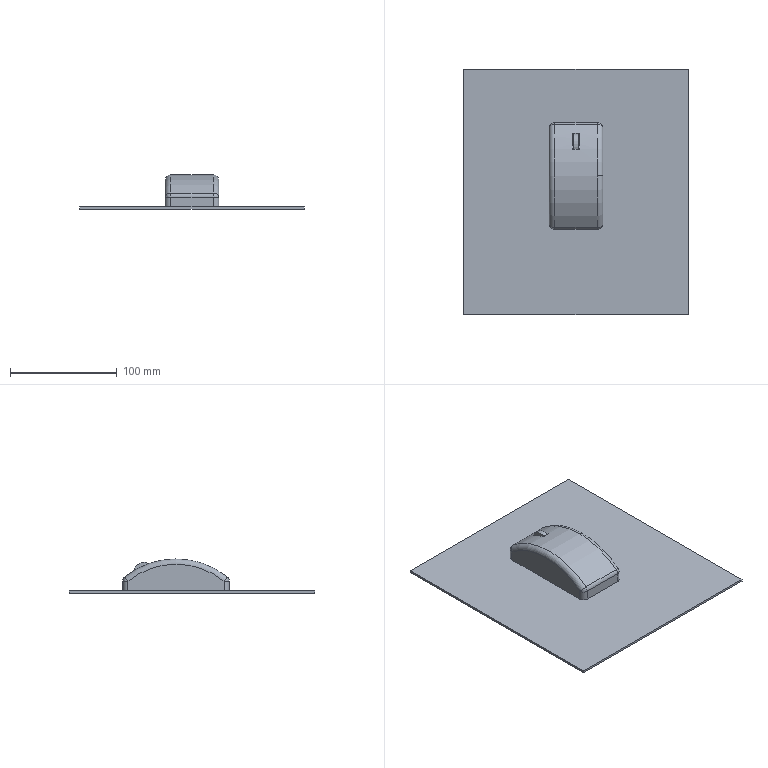Part | SolidWorks | features ICE 4, Fillet 2, Extrusion 1 | 1 solid | 32 faces | box 210 x 230 x 32 mm | volume 215921 mm3 | plane 17 | cylinder 8 | sphere 4 | torus 3 | commonest cylinder face diameters 10 x6 21 x1 153.572 x1
STEP:
#1=CARTESIAN_POINT('',(50.,50.,25.));
#2=VERTEX_POINT('',#1);
#3=CARTESIAN_POINT('',(50.,5.,9.145));
#4=VERTEX_POINT('',#3);
#5=CARTESIAN_POINT('',(50.,50.,-46.786));
#6=DIRECTION('',(1.,0.,0.));
#7=DIRECTION('',(0.,0.,1.));
#8=AXIS2_PLACEMENT_3D('',#5,#6,#7);
#9=CIRCLE('',#8,71.786);
#10=EDGE_CURVE('',#2,#4,#9,.T.);
#11=ORIENTED_EDGE('',*,*,#10,.F.);
#12=CARTESIAN_POINT('',(45.,50.,30.));
#13=VERTEX_POINT('',#12);
#14=CARTESIAN_POINT('',(45.,50.,25.));
#15=DIRECTION('',(0.,-1.,0.));
#16=DIRECTION('',(0.,0.,-1.));
#17=AXIS2_PLACEMENT_3D('',#14,#15,#16);
#18=CIRCLE('',#17,5.);
#19=EDGE_CURVE('',#2,#13,#18,.T.);
#20=ORIENTED_EDGE('',*,*,#19,.T.);
#21=CARTESIAN_POINT('',(45.,1.866,13.04));
#22=VERTEX_POINT('',#21);
#23=CARTESIAN_POINT('',(45.,50.,-46.786));
#24=DIRECTION('',(-1.,0.,0.));
#25=DIRECTION('',(0.,0.,1.));
#26=AXIS2_PLACEMENT_3D('',#23,#24,#25);
#27=CIRCLE('',#26,76.786);
#28=EDGE_CURVE('',#22,#13,#27,.T.);
#29=ORIENTED_EDGE('',*,*,#28,.F.);
#30=CARTESIAN_POINT('',(45.,5.,9.145));
#31=DIRECTION('',(0.,0.7791,0.6269));
#32=DIRECTION('',(0.,-0.6269,0.7791));
#33=AXIS2_PLACEMENT_3D('',#30,#31,#32);
#34=CIRCLE('',#33,5.);
#35=EDGE_CURVE('',#22,#4,#34,.T.);
#36=ORIENTED_EDGE('',*,*,#35,.T.);
#37=EDGE_LOOP('',(#11,#20,#29,#36));
#38=FACE_OUTER_BOUND('',#37,.T.);
#39=CARTESIAN_POINT('',(45.,50.,-46.786));
#40=DIRECTION('',(-1.,0.,0.));
#41=DIRECTION('',(0.,0.,1.));
#42=AXIS2_PLACEMENT_3D('',#39,#40,#41);
#43=TOROIDAL_SURFACE('',#42,71.786,5.);
#44=ADVANCED_FACE('',(#38),#43,.T.);
#45=CARTESIAN_POINT('',(23.,75.,25.703));
#46=VERTEX_POINT('',#45);
#47=CARTESIAN_POINT('',(27.,75.,25.703));
#48=VERTEX_POINT('',#47);
#49=CARTESIAN_POINT('',(23.,75.,25.703));
#50=DIRECTION('',(1.,0.,0.));
#51=VECTOR('',#50,1000.);
#52=LINE('',#49,#51);
#53=EDGE_CURVE('',#46,#48,#52,.T.);
#54=ORIENTED_EDGE('',*,*,#53,.F.);
#55=CARTESIAN_POINT('',(23.,75.,16.45));
#56=VERTEX_POINT('',#55);
#57=CARTESIAN_POINT('',(23.,75.,26.45));
#58=DIRECTION('',(0.,0.,-1.));
#59=VECTOR('',#58,1000.);
#60=LINE('',#57,#59);
#61=EDGE_CURVE('',#46,#56,#60,.T.);
#62=ORIENTED_EDGE('',*,*,#61,.T.);
#63=CARTESIAN_POINT('',(22.,75.,16.45));
#64=VERTEX_POINT('',#63);
#65=CARTESIAN_POINT('',(28.,75.,16.45));
#66=DIRECTION('',(-1.,0.,0.));
#67=VECTOR('',#66,1000.);
#68=LINE('',#65,#67);
#69=EDGE_CURVE('',#56,#64,#68,.T.);
#70=ORIENTED_EDGE('',*,*,#69,.T.);
#71=CARTESIAN_POINT('',(22.,75.,25.816));
#72=VERTEX_POINT('',#71);
#73=CARTESIAN_POINT('',(22.,75.,26.45));
#74=DIRECTION('',(0.,0.,-1.));
#75=VECTOR('',#74,1000.);
#76=LINE('',#73,#75);
#77=EDGE_CURVE('',#72,#64,#76,.T.);
#78=ORIENTED_EDGE('',*,*,#77,.F.);
#79=CARTESIAN_POINT('',(28.,75.,25.816));
#80=VERTEX_POINT('',#79);
#81=CARTESIAN_POINT('',(0.,75.,25.816));
#82=DIRECTION('',(1.,0.,0.));
#83=VECTOR('',#82,1000.);
#84=LINE('',#81,#83);
#85=EDGE_CURVE('',#72,#80,#84,.T.);
#86=ORIENTED_EDGE('',*,*,#85,.T.);
#87=CARTESIAN_POINT('',(28.,75.,16.45));
#88=VERTEX_POINT('',#87);
#89=CARTESIAN_POINT('',(28.,75.,26.45));
#90=DIRECTION('',(0.,0.,-1.));
#91=VECTOR('',#90,1000.);
#92=LINE('',#89,#91);
#93=EDGE_CURVE('',#80,#88,#92,.T.);
#94=ORIENTED_EDGE('',*,*,#93,.T.);
#95=CARTESIAN_POINT('',(27.,75.,16.45));
#96=VERTEX_POINT('',#95);
#97=CARTESIAN_POINT('',(28.,75.,16.45));
#98=DIRECTION('',(-1.,0.,0.));
#99=VECTOR('',#98,1000.);
#100=LINE('',#97,#99);
#101=EDGE_CURVE('',#88,#96,#100,.T.);
#102=ORIENTED_EDGE('',*,*,#101,.T.);
#103=CARTESIAN_POINT('',(27.,75.,26.45));
#104=DIRECTION('',(0.,0.,-1.));
#105=VECTOR('',#104,1000.);
#106=LINE('',#103,#105);
#107=EDGE_CURVE('',#48,#96,#106,.T.);
#108=ORIENTED_EDGE('',*,*,#107,.F.);
#109=EDGE_LOOP('',(#54,#62,#70,#78,#86,#94,#102,#108));
#110=FACE_OUTER_BOUND('',#109,.T.);
#111=CARTESIAN_POINT('',(28.,75.,26.45));
#112=DIRECTION('',(0.,1.,0.));
#113=DIRECTION('',(0.,0.,1.));
#114=AXIS2_PLACEMENT_3D('',#111,#112,#113);
#115=PLANE('',#114);
#116=ADVANCED_FACE('',(#110),#115,.T.);
#117=ORIENTED_EDGE('',*,*,#69,.F.);
#118=CARTESIAN_POINT('',(23.,89.997,16.45));
#119=VERTEX_POINT('',#118);
#120=CARTESIAN_POINT('',(23.,90.,16.45));
#121=DIRECTION('',(0.,1.,0.));
#122=VECTOR('',#121,1000.);
#123=LINE('',#120,#122);
#124=EDGE_CURVE('',#56,#119,#123,.T.);
#125=ORIENTED_EDGE('',*,*,#124,.T.);
#126=CARTESIAN_POINT('',(27.,89.997,16.45));
#127=VERTEX_POINT('',#126);
#128=CARTESIAN_POINT('',(23.,89.997,16.45));
#129=DIRECTION('',(-1.,0.,0.));
#130=VECTOR('',#129,1000.);
#131=LINE('',#128,#130);
#132=EDGE_CURVE('',#127,#119,#131,.T.);
#133=ORIENTED_EDGE('',*,*,#132,.F.);
#134=CARTESIAN_POINT('',(27.,90.,16.45));
#135=DIRECTION('',(0.,1.,0.));
#136=VECTOR('',#135,1000.);
#137=LINE('',#134,#136);
#138=EDGE_CURVE('',#96,#127,#137,.T.);
#139=ORIENTED_EDGE('',*,*,#138,.F.);
#140=ORIENTED_EDGE('',*,*,#101,.F.);
#141=CARTESIAN_POINT('',(28.,90.,16.45));
#142=VERTEX_POINT('',#141);
#143=CARTESIAN_POINT('',(28.,90.,16.45));
#144=DIRECTION('',(0.,1.,0.));
#145=VECTOR('',#144,1000.);
#146=LINE('',#143,#145);
#147=EDGE_CURVE('',#88,#142,#146,.T.);
#148=ORIENTED_EDGE('',*,*,#147,.T.);
#149=CARTESIAN_POINT('',(22.,90.,16.45));
#150=VERTEX_POINT('',#149);
#151=CARTESIAN_POINT('',(28.,90.,16.45));
#152=DIRECTION('',(-1.,0.,0.));
#153=VECTOR('',#152,1000.);
#154=LINE('',#151,#153);
#155=EDGE_CURVE('',#142,#150,#154,.T.);
#156=ORIENTED_EDGE('',*,*,#155,.T.);
#157=CARTESIAN_POINT('',(22.,90.,16.45));
#158=DIRECTION('',(0.,1.,0.));
#159=VECTOR('',#158,1000.);
#160=LINE('',#157,#159);
#161=EDGE_CURVE('',#64,#150,#160,.T.);
#162=ORIENTED_EDGE('',*,*,#161,.F.);
#163=EDGE_LOOP('',(#117,#125,#133,#139,#140,#148,#156,#162));
#164=FACE_OUTER_BOUND('',#163,.T.);
#165=CARTESIAN_POINT('',(28.,90.,16.45));
#166=DIRECTION('',(0.,0.,1.));
#167=DIRECTION('',(1.,0.,0.));
#168=AXIS2_PLACEMENT_3D('',#165,#166,#167);
#169=PLANE('',#168);
#170=ADVANCED_FACE('',(#164),#169,.T.);
#171=CARTESIAN_POINT('',(0.,5.,9.145));
#172=VERTEX_POINT('',#171);
#173=CARTESIAN_POINT('',(0.,95.,9.145));
#174=VERTEX_POINT('',#173);
#175=CARTESIAN_POINT('',(0.,50.,-46.786));
#176=DIRECTION('',(-1.,0.,0.));
#177=DIRECTION('',(0.,0.,-1.));
#178=AXIS2_PLACEMENT_3D('',#175,#176,#177);
#179=CIRCLE('',#178,71.786);
#180=EDGE_CURVE('',#172,#174,#179,.T.);
#181=ORIENTED_EDGE('',*,*,#180,.T.);
#182=CARTESIAN_POINT('',(0.,95.,0.));
#183=VERTEX_POINT('',#182);
#184=CARTESIAN_POINT('',(0.,95.,30.));
#185=DIRECTION('',(0.,0.,-1.));
#186=VECTOR('',#185,1000.);
#187=LINE('',#184,#186);
#188=EDGE_CURVE('',#174,#183,#187,.T.);
#189=ORIENTED_EDGE('',*,*,#188,.T.);
#190=CARTESIAN_POINT('',(0.,5.,0.));
#191=VERTEX_POINT('',#190);
#192=CARTESIAN_POINT('',(0.,0.,0.));
#193=DIRECTION('',(0.,-1.,0.));
#194=VECTOR('',#193,1000.);
#195=LINE('',#192,#194);
#196=EDGE_CURVE('',#183,#191,#195,.T.);
#197=ORIENTED_EDGE('',*,*,#196,.T.);
#198=CARTESIAN_POINT('',(0.,5.,30.));
#199=DIRECTION('',(0.,0.,1.));
#200=VECTOR('',#199,1000.);
#201=LINE('',#198,#200);
#202=EDGE_CURVE('',#191,#172,#201,.T.);
#203=ORIENTED_EDGE('',*,*,#202,.T.);
#204=EDGE_LOOP('',(#181,#189,#197,#203));
#205=FACE_OUTER_BOUND('',#204,.T.);
#206=CARTESIAN_POINT('',(0.,0.,30.));
#207=DIRECTION('',(1.,0.,0.));
#208=DIRECTION('',(0.,0.,-1.));
#209=AXIS2_PLACEMENT_3D('',#206,#207,#208);
#210=PLANE('',#209);
#211=ADVANCED_FACE('',(#205),#210,.F.);
#212=CARTESIAN_POINT('',(5.,0.,0.));
#213=VERTEX_POINT('',#212);
#214=CARTESIAN_POINT('',(45.,0.,0.));
#215=VERTEX_POINT('',#214);
#216=CARTESIAN_POINT('',(0.,0.,0.));
#217=DIRECTION('',(1.,0.,0.));
#218=VECTOR('',#217,1000.);
#219=LINE('',#216,#218);
#220=EDGE_CURVE('',#213,#215,#219,.T.);
#221=ORIENTED_EDGE('',*,*,#220,.T.);
#222=CARTESIAN_POINT('',(45.,0.,9.145));
#223=VERTEX_POINT('',#222);
#224=CARTESIAN_POINT('',(45.,0.,30.));
#225=DIRECTION('',(0.,0.,1.));
#226=VECTOR('',#225,1000.);
#227=LINE('',#224,#226);
#228=EDGE_CURVE('',#215,#223,#227,.T.);
#229=ORIENTED_EDGE('',*,*,#228,.T.);
#230=CARTESIAN_POINT('',(5.,0.,9.145));
#231=VERTEX_POINT('',#230);
#232=CARTESIAN_POINT('',(0.,0.,9.145));
#233=DIRECTION('',(-1.,0.,0.));
#234=VECTOR('',#233,1000.);
#235=LINE('',#232,#234);
#236=EDGE_CURVE('',#223,#231,#235,.T.);
#237=ORIENTED_EDGE('',*,*,#236,.T.);
#238=CARTESIAN_POINT('',(5.,0.,30.));
#239=DIRECTION('',(0.,0.,-1.));
#240=VECTOR('',#239,1000.);
#241=LINE('',#238,#240);
#242=EDGE_CURVE('',#231,#213,#241,.T.);
#243=ORIENTED_EDGE('',*,*,#242,.T.);
#244=EDGE_LOOP('',(#221,#229,#237,#243));
#245=FACE_OUTER_BOUND('',#244,.T.);
#246=CARTESIAN_POINT('',(0.,0.,30.));
#247=DIRECTION('',(0.,1.,0.));
#248=DIRECTION('',(0.,0.,1.));
#249=AXIS2_PLACEMENT_3D('',#246,#247,#248);
#250=PLANE('',#249);
#251=ADVANCED_FACE('',(#245),#250,.F.);
#252=CARTESIAN_POINT('',(50.,5.,0.));
#253=VERTEX_POINT('',#252);
#254=CARTESIAN_POINT('',(50.,95.,0.));
#255=VERTEX_POINT('',#254);
#256=CARTESIAN_POINT('',(50.,0.,0.));
#257=DIRECTION('',(0.,1.,0.));
#258=VECTOR('',#257,1000.);
#259=LINE('',#256,#258);
#260=EDGE_CURVE('',#253,#255,#259,.T.);
#261=ORIENTED_EDGE('',*,*,#260,.T.);
#262=CARTESIAN_POINT('',(50.,95.,9.145));
#263=VERTEX_POINT('',#262);
#264=CARTESIAN_POINT('',(50.,95.,30.));
#265=DIRECTION('',(0.,0.,1.));
#266=VECTOR('',#265,1000.);
#267=LINE('',#264,#266);
#268=EDGE_CURVE('',#255,#263,#267,.T.);
#269=ORIENTED_EDGE('',*,*,#268,.T.);
#270=CARTESIAN_POINT('',(50.,50.,-46.786));
#271=DIRECTION('',(1.,0.,0.));
#272=DIRECTION('',(0.,0.,1.));
#273=AXIS2_PLACEMENT_3D('',#270,#271,#272);
#274=CIRCLE('',#273,71.786);
#275=EDGE_CURVE('',#263,#2,#274,.T.);
#276=ORIENTED_EDGE('',*,*,#275,.T.);
#277=ORIENTED_EDGE('',*,*,#10,.T.);
#278=CARTESIAN_POINT('',(50.,5.,30.));
#279=DIRECTION('',(0.,0.,-1.));
#280=VECTOR('',#279,1000.);
#281=LINE('',#278,#280);
#282=EDGE_CURVE('',#4,#253,#281,.T.);
#283=ORIENTED_EDGE('',*,*,#282,.T.);
#284=EDGE_LOOP('',(#261,#269,#276,#277,#283));
#285=FACE_OUTER_BOUND('',#284,.T.);
#286=CARTESIAN_POINT('',(50.,0.,30.));
#287=DIRECTION('',(-1.,0.,0.));
#288=DIRECTION('',(0.,0.,1.));
#289=AXIS2_PLACEMENT_3D('',#286,#287,#288);
#290=PLANE('',#289);
#291=ADVANCED_FACE('',(#285),#290,.F.);
#292=CARTESIAN_POINT('',(45.,100.,0.));
#293=VERTEX_POINT('',#292);
#294=CARTESIAN_POINT('',(5.,100.,0.));
#295=VERTEX_POINT('',#294);
#296=CARTESIAN_POINT('',(0.,100.,0.));
#297=DIRECTION('',(-1.,0.,0.));
#298=VECTOR('',#297,1000.);
#299=LINE('',#296,#298);
#300=EDGE_CURVE('',#293,#295,#299,.T.);
#301=ORIENTED_EDGE('',*,*,#300,.T.);
#302=CARTESIAN_POINT('',(5.,100.,9.145));
#303=VERTEX_POINT('',#302);
#304=CARTESIAN_POINT('',(5.,100.,30.));
#305=DIRECTION('',(0.,0.,1.));
#306=VECTOR('',#305,1000.);
#307=LINE('',#304,#306);
#308=EDGE_CURVE('',#295,#303,#307,.T.);
#309=ORIENTED_EDGE('',*,*,#308,.T.);
#310=CARTESIAN_POINT('',(45.,100.,9.145));
#311=VERTEX_POINT('',#310);
#312=CARTESIAN_POINT('',(0.,100.,9.145));
#313=DIRECTION('',(1.,0.,0.));
#314=VECTOR('',#313,1000.);
#315=LINE('',#312,#314);
#316=EDGE_CURVE('',#303,#311,#315,.T.);
#317=ORIENTED_EDGE('',*,*,#316,.T.);
#318=CARTESIAN_POINT('',(45.,100.,30.));
#319=DIRECTION('',(0.,0.,-1.));
#320=VECTOR('',#319,1000.);
#321=LINE('',#318,#320);
#322=EDGE_CURVE('',#311,#293,#321,.T.);
#323=ORIENTED_EDGE('',*,*,#322,.T.);
#324=EDGE_LOOP('',(#301,#309,#317,#323));
#325=FACE_OUTER_BOUND('',#324,.T.);
#326=CARTESIAN_POINT('',(0.,100.,30.));
#327=DIRECTION('',(0.,-1.,0.));
#328=DIRECTION('',(0.,0.,-1.));
#329=AXIS2_PLACEMENT_3D('',#326,#327,#328);
#330=PLANE('',#329);
#331=ADVANCED_FACE('',(#325),#330,.F.);
#332=CARTESIAN_POINT('',(5.,98.134,13.04));
#333=VERTEX_POINT('',#332);
#334=CARTESIAN_POINT('',(5.,1.866,13.04));
#335=VERTEX_POINT('',#334);
#336=CARTESIAN_POINT('',(5.,50.,-46.786));
#337=DIRECTION('',(1.,0.,0.));
#338=DIRECTION('',(0.,0.,-1.));
#339=AXIS2_PLACEMENT_3D('',#336,#337,#338);
#340=CIRCLE('',#339,76.786);
#341=EDGE_CURVE('',#333,#335,#340,.T.);
#342=ORIENTED_EDGE('',*,*,#341,.T.);
#343=CARTESIAN_POINT('',(0.,1.866,13.04));
#344=DIRECTION('',(1.,0.,0.));
#345=VECTOR('',#344,1000.);
#346=LINE('',#343,#345);
#347=EDGE_CURVE('',#335,#22,#346,.T.);
#348=ORIENTED_EDGE('',*,*,#347,.T.);
#349=ORIENTED_EDGE('',*,*,#28,.T.);
#350=CARTESIAN_POINT('',(45.,98.134,13.04));
#351=VERTEX_POINT('',#350);
#352=CARTESIAN_POINT('',(45.,50.,-46.786));
#353=DIRECTION('',(-1.,0.,0.));
#354=DIRECTION('',(0.,0.,1.));
#355=AXIS2_PLACEMENT_3D('',#352,#353,#354);
#356=CIRCLE('',#355,76.786);
#357=EDGE_CURVE('',#13,#351,#356,.T.);
#358=ORIENTED_EDGE('',*,*,#357,.T.);
#359=CARTESIAN_POINT('',(0.,98.134,13.04));
#360=DIRECTION('',(-1.,0.,0.));
#361=VECTOR('',#360,1000.);
#362=LINE('',#359,#361);
#363=EDGE_CURVE('',#351,#333,#362,.T.);
#364=ORIENTED_EDGE('',*,*,#363,.T.);
#365=EDGE_LOOP('',(#342,#348,#349,#358,#364));
#366=FACE_OUTER_BOUND('',#365,.T.);
#367=CARTESIAN_POINT('',(28.,90.,18.759));
#368=VERTEX_POINT('',#367);
#369=CARTESIAN_POINT('',(22.,90.,18.759));
#370=VERTEX_POINT('',#369);
#371=CARTESIAN_POINT('',(0.,90.,18.759));
#372=DIRECTION('',(-1.,0.,0.));
#373=VECTOR('',#372,1000.);
#374=LINE('',#371,#373);
#375=EDGE_CURVE('',#368,#370,#374,.T.);
#376=ORIENTED_EDGE('',*,*,#375,.F.);
#377=CARTESIAN_POINT('',(28.,50.,-46.786));
#378=DIRECTION('',(1.,0.,0.));
#379=DIRECTION('',(0.,0.,-1.));
#380=AXIS2_PLACEMENT_3D('',#377,#378,#379);
#381=CIRCLE('',#380,76.786);
#382=EDGE_CURVE('',#368,#80,#381,.T.);
#383=ORIENTED_EDGE('',*,*,#382,.T.);
#384=ORIENTED_EDGE('',*,*,#85,.F.);
#385=CARTESIAN_POINT('',(22.,50.,-46.786));
#386=DIRECTION('',(1.,0.,0.));
#387=DIRECTION('',(0.,0.,-1.));
#388=AXIS2_PLACEMENT_3D('',#385,#386,#387);
#389=CIRCLE('',#388,76.786);
#390=EDGE_CURVE('',#370,#72,#389,.T.);
#391=ORIENTED_EDGE('',*,*,#390,.F.);
#392=EDGE_LOOP('',(#376,#383,#384,#391));
#393=FACE_BOUND('',#392,.T.);
#394=CARTESIAN_POINT('',(0.,50.,-46.786));
#395=DIRECTION('',(1.,0.,0.));
#396=DIRECTION('',(0.,0.,-1.));
#397=AXIS2_PLACEMENT_3D('',#394,#395,#396);
#398=CYLINDRICAL_SURFACE('',#397,76.786);
#399=ADVANCED_FACE('',(#366,#393),#398,.T.);
#400=ORIENTED_EDGE('',*,*,#375,.T.);
#401=CARTESIAN_POINT('',(22.,90.,26.45));
#402=DIRECTION('',(0.,0.,1.));
#403=VECTOR('',#402,1000.);
#404=LINE('',#401,#403);
#405=EDGE_CURVE('',#150,#370,#404,.T.);
#406=ORIENTED_EDGE('',*,*,#405,.F.);
#407=ORIENTED_EDGE('',*,*,#155,.F.);
#408=CARTESIAN_POINT('',(28.,90.,26.45));
#409=DIRECTION('',(0.,0.,1.));
#410=VECTOR('',#409,1000.);
#411=LINE('',#408,#410);
#412=EDGE_CURVE('',#142,#368,#411,.T.);
#413=ORIENTED_EDGE('',*,*,#412,.T.);
#414=EDGE_LOOP('',(#400,#406,#407,#413));
#415=FACE_OUTER_BOUND('',#414,.T.);
#416=CARTESIAN_POINT('',(28.,90.,26.45));
#417=DIRECTION('',(0.,-1.,0.));
#418=DIRECTION('',(0.,0.,-1.));
#419=AXIS2_PLACEMENT_3D('',#416,#417,#418);
#420=PLANE('',#419);
#421=ADVANCED_FACE('',(#415),#420,.T.);
#422=ORIENTED_EDGE('',*,*,#412,.F.);
#423=ORIENTED_EDGE('',*,*,#147,.F.);
#424=ORIENTED_EDGE('',*,*,#93,.F.);
#425=ORIENTED_EDGE('',*,*,#382,.F.);
#426=EDGE_LOOP('',(#422,#423,#424,#425));
#427=FACE_OUTER_BOUND('',#426,.T.);
#428=CARTESIAN_POINT('',(28.,75.,26.45));
#429=DIRECTION('',(1.,0.,0.));
#430=DIRECTION('',(0.,0.,-1.));
#431=AXIS2_PLACEMENT_3D('',#428,#429,#430);
#432=PLANE('',#431);
#433=ADVANCED_FACE('',(#427),#432,.F.);
#434=ORIENTED_EDGE('',*,*,#390,.T.);
#435=ORIENTED_EDGE('',*,*,#77,.T.);
#436=ORIENTED_EDGE('',*,*,#161,.T.);
#437=ORIENTED_EDGE('',*,*,#405,.T.);
#438=EDGE_LOOP('',(#434,#435,#436,#437));
#439=FACE_OUTER_BOUND('',#438,.T.);
#440=CARTESIAN_POINT('',(22.,75.,26.45));
#441=DIRECTION('',(1.,0.,0.));
#442=DIRECTION('',(0.,0.,-1.));
#443=AXIS2_PLACEMENT_3D('',#440,#441,#442);
#444=PLANE('',#443);
#445=ADVANCED_FACE('',(#439),#444,.T.);
#446=CARTESIAN_POINT('',(23.,79.5,16.217));
#447=DIRECTION('',(1.,0.,0.));
#448=DIRECTION('',(0.,0.,-1.));
#449=AXIS2_PLACEMENT_3D('',#446,#447,#448);
#450=CIRCLE('',#449,10.5);
#451=EDGE_CURVE('',#119,#46,#450,.T.);
#452=ORIENTED_EDGE('',*,*,#451,.T.);
#453=ORIENTED_EDGE('',*,*,#53,.T.);
#454=CARTESIAN_POINT('',(27.,79.5,16.217));
#455=DIRECTION('',(1.,0.,0.));
#456=DIRECTION('',(0.,0.,-1.));
#457=AXIS2_PLACEMENT_3D('',#454,#455,#456);
#458=CIRCLE('',#457,10.5);
#459=EDGE_CURVE('',#127,#48,#458,.T.);
#460=ORIENTED_EDGE('',*,*,#459,.F.);
#461=ORIENTED_EDGE('',*,*,#132,.T.);
#462=EDGE_LOOP('',(#452,#453,#460,#461));
#463=FACE_OUTER_BOUND('',#462,.T.);
#464=CARTESIAN_POINT('',(23.,79.5,16.217));
#465=DIRECTION('',(1.,0.,0.));
#466=DIRECTION('',(0.,0.,-1.));
#467=AXIS2_PLACEMENT_3D('',#464,#465,#466);
#468=CYLINDRICAL_SURFACE('',#467,10.5);
#469=ADVANCED_FACE('',(#463),#468,.T.);
#470=ORIENTED_EDGE('',*,*,#61,.F.);
#471=ORIENTED_EDGE('',*,*,#451,.F.);
#472=ORIENTED_EDGE('',*,*,#124,.F.);
#473=EDGE_LOOP('',(#470,#471,#472));
#474=FACE_OUTER_BOUND('',#473,.T.);
#475=CARTESIAN_POINT('',(23.,79.5,16.217));
#476=DIRECTION('',(1.,0.,0.));
#477=DIRECTION('',(0.,0.,-1.));
#478=AXIS2_PLACEMENT_3D('',#475,#476,#477);
#479=PLANE('',#478);
#480=ADVANCED_FACE('',(#474),#479,.F.);
#481=ORIENTED_EDGE('',*,*,#459,.T.);
#482=ORIENTED_EDGE('',*,*,#107,.T.);
#483=ORIENTED_EDGE('',*,*,#138,.T.);
#484=EDGE_LOOP('',(#481,#482,#483));
#485=FACE_OUTER_BOUND('',#484,.T.);
#486=CARTESIAN_POINT('',(27.,79.5,16.217));
#487=DIRECTION('',(1.,0.,0.));
#488=DIRECTION('',(0.,0.,-1.));
#489=AXIS2_PLACEMENT_3D('',#486,#487,#488);
#490=PLANE('',#489);
#491=ADVANCED_FACE('',(#485),#490,.T.);
#492=ORIENTED_EDGE('',*,*,#316,.F.);
#493=CARTESIAN_POINT('',(5.,95.,9.145));
#494=DIRECTION('',(1.,0.,0.));
#495=DIRECTION('',(0.,0.,-1.));
#496=AXIS2_PLACEMENT_3D('',#493,#494,#495);
#497=CIRCLE('',#496,5.);
#498=EDGE_CURVE('',#303,#333,#497,.T.);
#499=ORIENTED_EDGE('',*,*,#498,.T.);
#500=ORIENTED_EDGE('',*,*,#363,.F.);
#501=CARTESIAN_POINT('',(45.,95.,9.145));
#502=DIRECTION('',(-1.,0.,0.));
#503=DIRECTION('',(0.,0.,-1.));
#504=AXIS2_PLACEMENT_3D('',#501,#502,#503);
#505=CIRCLE('',#504,5.);
#506=EDGE_CURVE('',#351,#311,#505,.T.);
#507=ORIENTED_EDGE('',*,*,#506,.T.);
#508=EDGE_LOOP('',(#492,#499,#500,#507));
#509=FACE_OUTER_BOUND('',#508,.T.);
#510=CARTESIAN_POINT('',(0.,95.,9.145));
#511=DIRECTION('',(1.,0.,0.));
#512=DIRECTION('',(0.,0.,-1.));
#513=AXIS2_PLACEMENT_3D('',#510,#511,#512);
#514=CYLINDRICAL_SURFACE('',#513,5.);
#515=ADVANCED_FACE('',(#509),#514,.T.);
#516=ORIENTED_EDGE('',*,*,#19,.F.);
#517=ORIENTED_EDGE('',*,*,#275,.F.);
#518=CARTESIAN_POINT('',(45.,95.,9.145));
#519=DIRECTION('',(0.,-0.7791,0.6269));
#520=DIRECTION('',(0.,0.6269,0.7791));
#521=AXIS2_PLACEMENT_3D('',#518,#519,#520);
#522=CIRCLE('',#521,5.);
#523=EDGE_CURVE('',#263,#351,#522,.T.);
#524=ORIENTED_EDGE('',*,*,#523,.T.);
#525=ORIENTED_EDGE('',*,*,#357,.F.);
#526=EDGE_LOOP('',(#516,#517,#524,#525));
#527=FACE_OUTER_BOUND('',#526,.T.);
#528=CARTESIAN_POINT('',(45.,50.,-46.786));
#529=DIRECTION('',(-1.,0.,0.));
#530=DIRECTION('',(0.,0.,1.));
#531=AXIS2_PLACEMENT_3D('',#528,#529,#530);
#532=TOROIDAL_SURFACE('',#531,71.786,5.);
#533=ADVANCED_FACE('',(#527),#532,.T.);
#534=ORIENTED_EDGE('',*,*,#341,.F.);
#535=CARTESIAN_POINT('',(5.,95.,9.145));
#536=DIRECTION('',(0.,-0.7791,0.6269));
#537=DIRECTION('',(0.,-0.6269,-0.7791));
#538=AXIS2_PLACEMENT_3D('',#535,#536,#537);
#539=CIRCLE('',#538,5.);
#540=EDGE_CURVE('',#333,#174,#539,.T.);
#541=ORIENTED_EDGE('',*,*,#540,.T.);
#542=ORIENTED_EDGE('',*,*,#180,.F.);
#543=CARTESIAN_POINT('',(5.,5.,9.145));
#544=DIRECTION('',(0.,0.7791,0.6269));
#545=DIRECTION('',(0.,0.6269,-0.7791));
#546=AXIS2_PLACEMENT_3D('',#543,#544,#545);
#547=CIRCLE('',#546,5.);
#548=EDGE_CURVE('',#172,#335,#547,.T.);
#549=ORIENTED_EDGE('',*,*,#548,.T.);
#550=EDGE_LOOP('',(#534,#541,#542,#549));
#551=FACE_OUTER_BOUND('',#550,.T.);
#552=CARTESIAN_POINT('',(5.,50.,-46.786));
#553=DIRECTION('',(1.,0.,0.));
#554=DIRECTION('',(0.,0.,-1.));
#555=AXIS2_PLACEMENT_3D('',#552,#553,#554);
#556=TOROIDAL_SURFACE('',#555,71.786,5.);
#557=ADVANCED_FACE('',(#551),#556,.T.);
#558=ORIENTED_EDGE('',*,*,#236,.F.);
#559=CARTESIAN_POINT('',(45.,5.,9.145));
#560=DIRECTION('',(-1.,0.,0.));
#561=DIRECTION('',(0.,0.,-1.));
#562=AXIS2_PLACEMENT_3D('',#559,#560,#561);
#563=CIRCLE('',#562,5.);
#564=EDGE_CURVE('',#223,#22,#563,.T.);
#565=ORIENTED_EDGE('',*,*,#564,.T.);
#566=ORIENTED_EDGE('',*,*,#347,.F.);
#567=CARTESIAN_POINT('',(5.,5.,9.145));
#568=DIRECTION('',(1.,0.,0.));
#569=DIRECTION('',(0.,0.,-1.));
#570=AXIS2_PLACEMENT_3D('',#567,#568,#569);
#571=CIRCLE('',#570,5.);
#572=EDGE_CURVE('',#335,#231,#571,.T.);
#573=ORIENTED_EDGE('',*,*,#572,.T.);
#574=EDGE_LOOP('',(#558,#565,#566,#573));
#575=FACE_OUTER_BOUND('',#574,.T.);
#576=CARTESIAN_POINT('',(0.,5.,9.145));
#577=DIRECTION('',(1.,0.,0.));
#578=DIRECTION('',(0.,0.,-1.));
#579=AXIS2_PLACEMENT_3D('',#576,#577,#578);
#580=CYLINDRICAL_SURFACE('',#579,5.);
#581=ADVANCED_FACE('',(#575),#580,.T.);
#582=CARTESIAN_POINT('',(5.,95.,9.145));
#583=DIRECTION('',(0.,0.,1.));
#584=DIRECTION('',(1.,0.,0.));
#585=AXIS2_PLACEMENT_3D('',#582,#583,#584);
#586=CIRCLE('',#585,5.);
#587=EDGE_CURVE('',#303,#174,#586,.T.);
#588=ORIENTED_EDGE('',*,*,#587,.F.);
#589=ORIENTED_EDGE('',*,*,#308,.F.);
#590=CARTESIAN_POINT('',(5.,95.,0.));
#591=DIRECTION('',(0.,0.,-1.));
#592=DIRECTION('',(-1.,0.,0.));
#593=AXIS2_PLACEMENT_3D('',#590,#591,#592);
#594=CIRCLE('',#593,5.);
#595=EDGE_CURVE('',#183,#295,#594,.T.);
#596=ORIENTED_EDGE('',*,*,#595,.F.);
#597=ORIENTED_EDGE('',*,*,#188,.F.);
#598=EDGE_LOOP('',(#588,#589,#596,#597));
#599=FACE_OUTER_BOUND('',#598,.T.);
#600=CARTESIAN_POINT('',(5.,95.,30.));
#601=DIRECTION('',(0.,0.,-1.));
#602=DIRECTION('',(-1.,0.,0.));
#603=AXIS2_PLACEMENT_3D('',#600,#601,#602);
#604=CYLINDRICAL_SURFACE('',#603,5.);
#605=ADVANCED_FACE('',(#599),#604,.T.);
#606=ORIENTED_EDGE('',*,*,#540,.F.);
#607=ORIENTED_EDGE('',*,*,#498,.F.);
#608=ORIENTED_EDGE('',*,*,#587,.T.);
#609=EDGE_LOOP('',(#606,#607,#608));
#610=FACE_OUTER_BOUND('',#609,.T.);
#611=CARTESIAN_POINT('',(5.,95.,9.145));
#612=DIRECTION('',(0.,1.,0.));
#613=DIRECTION('',(1.,0.,0.));
#614=AXIS2_PLACEMENT_3D('',#611,#612,#613);
#615=SPHERICAL_SURFACE('',#614,5.);
#616=ADVANCED_FACE('',(#610),#615,.T.);
#617=CARTESIAN_POINT('',(45.,95.,9.145));
#618=DIRECTION('',(0.,0.,1.));
#619=DIRECTION('',(1.,0.,0.));
#620=AXIS2_PLACEMENT_3D('',#617,#618,#619);
#621=CIRCLE('',#620,5.);
#622=EDGE_CURVE('',#263,#311,#621,.T.);
#623=ORIENTED_EDGE('',*,*,#622,.F.);
#624=ORIENTED_EDGE('',*,*,#268,.F.);
#625=CARTESIAN_POINT('',(45.,95.,0.));
#626=DIRECTION('',(0.,0.,-1.));
#627=DIRECTION('',(-1.,0.,0.));
#628=AXIS2_PLACEMENT_3D('',#625,#626,#627);
#629=CIRCLE('',#628,5.);
#630=EDGE_CURVE('',#293,#255,#629,.T.);
#631=ORIENTED_EDGE('',*,*,#630,.F.);
#632=ORIENTED_EDGE('',*,*,#322,.F.);
#633=EDGE_LOOP('',(#623,#624,#631,#632));
#634=FACE_OUTER_BOUND('',#633,.T.);
#635=CARTESIAN_POINT('',(45.,95.,30.));
#636=DIRECTION('',(0.,0.,-1.));
#637=DIRECTION('',(-1.,0.,0.));
#638=AXIS2_PLACEMENT_3D('',#635,#636,#637);
#639=CYLINDRICAL_SURFACE('',#638,5.);
#640=ADVANCED_FACE('',(#634),#639,.T.);
#641=ORIENTED_EDGE('',*,*,#622,.T.);
#642=ORIENTED_EDGE('',*,*,#506,.F.);
#643=ORIENTED_EDGE('',*,*,#523,.F.);
#644=EDGE_LOOP('',(#641,#642,#643));
#645=FACE_OUTER_BOUND('',#644,.T.);
#646=CARTESIAN_POINT('',(45.,95.,9.145));
#647=DIRECTION('',(0.,1.,0.));
#648=DIRECTION('',(1.,0.,0.));
#649=AXIS2_PLACEMENT_3D('',#646,#647,#648);
#650=SPHERICAL_SURFACE('',#649,5.);
#651=ADVANCED_FACE('',(#645),#650,.T.);
#652=CARTESIAN_POINT('',(45.,5.,9.145));
#653=DIRECTION('',(0.,0.,1.));
#654=DIRECTION('',(1.,0.,0.));
#655=AXIS2_PLACEMENT_3D('',#652,#653,#654);
#656=CIRCLE('',#655,5.);
#657=EDGE_CURVE('',#223,#4,#656,.T.);
#658=ORIENTED_EDGE('',*,*,#657,.F.);
#659=ORIENTED_EDGE('',*,*,#228,.F.);
#660=CARTESIAN_POINT('',(45.,5.,0.));
#661=DIRECTION('',(0.,0.,-1.));
#662=DIRECTION('',(-1.,0.,0.));
#663=AXIS2_PLACEMENT_3D('',#660,#661,#662);
#664=CIRCLE('',#663,5.);
#665=EDGE_CURVE('',#253,#215,#664,.T.);
#666=ORIENTED_EDGE('',*,*,#665,.F.);
#667=ORIENTED_EDGE('',*,*,#282,.F.);
#668=EDGE_LOOP('',(#658,#659,#666,#667));
#669=FACE_OUTER_BOUND('',#668,.T.);
#670=CARTESIAN_POINT('',(45.,5.,30.));
#671=DIRECTION('',(0.,0.,-1.));
#672=DIRECTION('',(-1.,0.,0.));
#673=AXIS2_PLACEMENT_3D('',#670,#671,#672);
#674=CYLINDRICAL_SURFACE('',#673,5.);
#675=ADVANCED_FACE('',(#669),#674,.T.);
#676=ORIENTED_EDGE('',*,*,#657,.T.);
#677=ORIENTED_EDGE('',*,*,#35,.F.);
#678=ORIENTED_EDGE('',*,*,#564,.F.);
#679=EDGE_LOOP('',(#676,#677,#678));
#680=FACE_OUTER_BOUND('',#679,.T.);
#681=CARTESIAN_POINT('',(45.,5.,9.145));
#682=DIRECTION('',(0.,1.,0.));
#683=DIRECTION('',(1.,0.,0.));
#684=AXIS2_PLACEMENT_3D('',#681,#682,#683);
#685=SPHERICAL_SURFACE('',#684,5.);
#686=ADVANCED_FACE('',(#680),#685,.T.);
#687=CARTESIAN_POINT('',(5.,5.,9.145));
#688=DIRECTION('',(0.,0.,1.));
#689=DIRECTION('',(0.,-1.,0.));
#690=AXIS2_PLACEMENT_3D('',#687,#688,#689);
#691=CIRCLE('',#690,5.);
#692=EDGE_CURVE('',#172,#231,#691,.T.);
#693=ORIENTED_EDGE('',*,*,#692,.F.);
#694=ORIENTED_EDGE('',*,*,#202,.F.);
#695=CARTESIAN_POINT('',(5.,5.,0.));
#696=DIRECTION('',(0.,0.,-1.));
#697=DIRECTION('',(-1.,0.,0.));
#698=AXIS2_PLACEMENT_3D('',#695,#696,#697);
#699=CIRCLE('',#698,5.);
#700=EDGE_CURVE('',#213,#191,#699,.T.);
#701=ORIENTED_EDGE('',*,*,#700,.F.);
#702=ORIENTED_EDGE('',*,*,#242,.F.);
#703=EDGE_LOOP('',(#693,#694,#701,#702));
#704=FACE_OUTER_BOUND('',#703,.T.);
#705=CARTESIAN_POINT('',(5.,5.,30.));
#706=DIRECTION('',(0.,0.,-1.));
#707=DIRECTION('',(-1.,0.,0.));
#708=AXIS2_PLACEMENT_3D('',#705,#706,#707);
#709=CYLINDRICAL_SURFACE('',#708,5.);
#710=ADVANCED_FACE('',(#704),#709,.T.);
#711=ORIENTED_EDGE('',*,*,#572,.F.);
#712=ORIENTED_EDGE('',*,*,#548,.F.);
#713=ORIENTED_EDGE('',*,*,#692,.T.);
#714=EDGE_LOOP('',(#711,#712,#713));
#715=FACE_OUTER_BOUND('',#714,.T.);
#716=CARTESIAN_POINT('',(5.,5.,9.145));
#717=DIRECTION('',(0.,1.,0.));
#718=DIRECTION('',(1.,0.,0.));
#719=AXIS2_PLACEMENT_3D('',#716,#717,#718);
#720=SPHERICAL_SURFACE('',#719,5.);
#721=ADVANCED_FACE('',(#715),#720,.T.);
#722=CARTESIAN_POINT('',(130.,150.,0.));
#723=VERTEX_POINT('',#722);
#724=CARTESIAN_POINT('',(130.,-80.,0.));
#725=VERTEX_POINT('',#724);
#726=CARTESIAN_POINT('',(130.,150.,0.));
#727=DIRECTION('',(0.,-1.,0.));
#728=VECTOR('',#727,1000.);
#729=LINE('',#726,#728);
#730=EDGE_CURVE('',#723,#725,#729,.T.);
#731=ORIENTED_EDGE('',*,*,#730,.T.);
#732=CARTESIAN_POINT('',(130.,-80.,-2.));
#733=VERTEX_POINT('',#732);
#734=CARTESIAN_POINT('',(130.,-80.,-2.));
#735=DIRECTION('',(0.,0.,1.));
#736=VECTOR('',#735,1000.);
#737=LINE('',#734,#736);
#738=EDGE_CURVE('',#733,#725,#737,.T.);
#739=ORIENTED_EDGE('',*,*,#738,.F.);
#740=CARTESIAN_POINT('',(130.,150.,-2.));
#741=VERTEX_POINT('',#740);
#742=CARTESIAN_POINT('',(130.,150.,-2.));
#743=DIRECTION('',(0.,-1.,0.));
#744=VECTOR('',#743,1000.);
#745=LINE('',#742,#744);
#746=EDGE_CURVE('',#741,#733,#745,.T.);
#747=ORIENTED_EDGE('',*,*,#746,.F.);
#748=CARTESIAN_POINT('',(130.,150.,-2.));
#749=DIRECTION('',(0.,0.,1.));
#750=VECTOR('',#749,1000.);
#751=LINE('',#748,#750);
#752=EDGE_CURVE('',#741,#723,#751,.T.);
#753=ORIENTED_EDGE('',*,*,#752,.T.);
#754=EDGE_LOOP('',(#731,#739,#747,#753));
#755=FACE_OUTER_BOUND('',#754,.T.);
#756=CARTESIAN_POINT('',(130.,150.,-2.));
#757=DIRECTION('',(-1.,0.,0.));
#758=DIRECTION('',(0.,-1.,0.));
#759=AXIS2_PLACEMENT_3D('',#756,#757,#758);
#760=PLANE('',#759);
#761=ADVANCED_FACE('',(#755),#760,.F.);
#762=CARTESIAN_POINT('',(-80.,-80.,0.));
#763=VERTEX_POINT('',#762);
#764=CARTESIAN_POINT('',(130.,-80.,0.));
#765=DIRECTION('',(-1.,0.,0.));
#766=VECTOR('',#765,1000.);
#767=LINE('',#764,#766);
#768=EDGE_CURVE('',#725,#763,#767,.T.);
#769=ORIENTED_EDGE('',*,*,#768,.T.);
#770=CARTESIAN_POINT('',(-80.,-80.,-2.));
#771=VERTEX_POINT('',#770);
#772=CARTESIAN_POINT('',(-80.,-80.,-2.));
#773=DIRECTION('',(0.,0.,1.));
#774=VECTOR('',#773,1000.);
#775=LINE('',#772,#774);
#776=EDGE_CURVE('',#771,#763,#775,.T.);
#777=ORIENTED_EDGE('',*,*,#776,.F.);
#778=CARTESIAN_POINT('',(130.,-80.,-2.));
#779=DIRECTION('',(-1.,0.,0.));
#780=VECTOR('',#779,1000.);
#781=LINE('',#778,#780);
#782=EDGE_CURVE('',#733,#771,#781,.T.);
#783=ORIENTED_EDGE('',*,*,#782,.F.);
#784=ORIENTED_EDGE('',*,*,#738,.T.);
#785=EDGE_LOOP('',(#769,#777,#783,#784));
#786=FACE_OUTER_BOUND('',#785,.T.);
#787=CARTESIAN_POINT('',(130.,-80.,-2.));
#788=DIRECTION('',(0.,1.,0.));
#789=DIRECTION('',(0.,0.,1.));
#790=AXIS2_PLACEMENT_3D('',#787,#788,#789);
#791=PLANE('',#790);
#792=ADVANCED_FACE('',(#786),#791,.F.);
#793=CARTESIAN_POINT('',(-80.,150.,0.));
#794=VERTEX_POINT('',#793);
#795=CARTESIAN_POINT('',(-80.,150.,0.));
#796=DIRECTION('',(0.,1.,0.));
#797=VECTOR('',#796,1000.);
#798=LINE('',#795,#797);
#799=EDGE_CURVE('',#763,#794,#798,.T.);
#800=ORIENTED_EDGE('',*,*,#799,.T.);
#801=CARTESIAN_POINT('',(-80.,150.,-2.));
#802=VERTEX_POINT('',#801);
#803=CARTESIAN_POINT('',(-80.,150.,-2.));
#804=DIRECTION('',(0.,0.,1.));
#805=VECTOR('',#804,1000.);
#806=LINE('',#803,#805);
#807=EDGE_CURVE('',#802,#794,#806,.T.);
#808=ORIENTED_EDGE('',*,*,#807,.F.);
#809=CARTESIAN_POINT('',(-80.,150.,-2.));
#810=DIRECTION('',(0.,1.,0.));
#811=VECTOR('',#810,1000.);
#812=LINE('',#809,#811);
#813=EDGE_CURVE('',#771,#802,#812,.T.);
#814=ORIENTED_EDGE('',*,*,#813,.F.);
#815=ORIENTED_EDGE('',*,*,#776,.T.);
#816=EDGE_LOOP('',(#800,#808,#814,#815));
#817=FACE_OUTER_BOUND('',#816,.T.);
#818=CARTESIAN_POINT('',(-80.,150.,-2.));
#819=DIRECTION('',(1.,0.,0.));
#820=DIRECTION('',(0.,1.,0.));
#821=AXIS2_PLACEMENT_3D('',#818,#819,#820);
#822=PLANE('',#821);
#823=ADVANCED_FACE('',(#817),#822,.F.);
#824=CARTESIAN_POINT('',(130.,150.,0.));
#825=DIRECTION('',(1.,0.,0.));
#826=VECTOR('',#825,1000.);
#827=LINE('',#824,#826);
#828=EDGE_CURVE('',#794,#723,#827,.T.);
#829=ORIENTED_EDGE('',*,*,#828,.T.);
#830=ORIENTED_EDGE('',*,*,#752,.F.);
#831=CARTESIAN_POINT('',(130.,150.,-2.));
#832=DIRECTION('',(1.,0.,0.));
#833=VECTOR('',#832,1000.);
#834=LINE('',#831,#833);
#835=EDGE_CURVE('',#802,#741,#834,.T.);
#836=ORIENTED_EDGE('',*,*,#835,.F.);
#837=ORIENTED_EDGE('',*,*,#807,.T.);
#838=EDGE_LOOP('',(#829,#830,#836,#837));
#839=FACE_OUTER_BOUND('',#838,.T.);
#840=CARTESIAN_POINT('',(130.,150.,-2.));
#841=DIRECTION('',(0.,-1.,0.));
#842=DIRECTION('',(0.,0.,-1.));
#843=AXIS2_PLACEMENT_3D('',#840,#841,#842);
#844=PLANE('',#843);
#845=ADVANCED_FACE('',(#839),#844,.F.);
#846=ORIENTED_EDGE('',*,*,#746,.T.);
#847=ORIENTED_EDGE('',*,*,#782,.T.);
#848=ORIENTED_EDGE('',*,*,#813,.T.);
#849=ORIENTED_EDGE('',*,*,#835,.T.);
#850=EDGE_LOOP('',(#846,#847,#848,#849));
#851=FACE_OUTER_BOUND('',#850,.T.);
#852=CARTESIAN_POINT('',(130.,-80.,-2.));
#853=DIRECTION('',(0.,0.,-1.));
#854=DIRECTION('',(-1.,0.,0.));
#855=AXIS2_PLACEMENT_3D('',#852,#853,#854);
#856=PLANE('',#855);
#857=ADVANCED_FACE('',(#851),#856,.T.);
#858=ORIENTED_EDGE('',*,*,#630,.T.);
#859=ORIENTED_EDGE('',*,*,#260,.F.);
#860=ORIENTED_EDGE('',*,*,#665,.T.);
#861=ORIENTED_EDGE('',*,*,#220,.F.);
#862=ORIENTED_EDGE('',*,*,#700,.T.);
#863=ORIENTED_EDGE('',*,*,#196,.F.);
#864=ORIENTED_EDGE('',*,*,#595,.T.);
#865=ORIENTED_EDGE('',*,*,#300,.F.);
#866=EDGE_LOOP('',(#858,#859,#860,#861,#862,#863,#864,#865));
#867=FACE_BOUND('',#866,.T.);
#868=ORIENTED_EDGE('',*,*,#730,.F.);
#869=ORIENTED_EDGE('',*,*,#828,.F.);
#870=ORIENTED_EDGE('',*,*,#799,.F.);
#871=ORIENTED_EDGE('',*,*,#768,.F.);
#872=EDGE_LOOP('',(#868,#869,#870,#871));
#873=FACE_OUTER_BOUND('',#872,.T.);
#874=CARTESIAN_POINT('',(130.,-80.,0.));
#875=DIRECTION('',(0.,0.,-1.));
#876=DIRECTION('',(-1.,0.,0.));
#877=AXIS2_PLACEMENT_3D('',#874,#875,#876);
#878=PLANE('',#877);
#879=ADVANCED_FACE('',(#867,#873),#878,.F.);
#880=CLOSED_SHELL('',(#44,#116,#170,#211,#251,#291,#331,#399,#421,#433,#445,#469,#480,#491,#515,#533,#557,#581,#605,#616,#640,#651,#675,#686,#710,#721,#761,#792,#823,#845,#857,#879));
#881=MANIFOLD_SOLID_BREP('',#880);
#882=CARTESIAN_POINT('',(0.,0.,0.));
#883=DIRECTION('',(0.,0.,1.));
#884=DIRECTION('',(1.,0.,0.));
#885=AXIS2_PLACEMENT_3D('',#882,#883,#884);
#886=(LENGTH_UNIT()NAMED_UNIT(*)SI_UNIT(.MILLI.,.METRE.));
#887=UNCERTAINTY_MEASURE_WITH_UNIT(LENGTH_MEASURE(0.00001),#886,'','');
#888=(NAMED_UNIT(*)PLANE_ANGLE_UNIT()SI_UNIT($,.RADIAN.));
#889=(NAMED_UNIT(*)SI_UNIT($,.STERADIAN.)SOLID_ANGLE_UNIT());
#890=(GEOMETRIC_REPRESENTATION_CONTEXT(3)GLOBAL_UNCERTAINTY_ASSIGNED_CONTEXT((#887))GLOBAL_UNIT_ASSIGNED_CONTEXT((#886,#888,#889))REPRESENTATION_CONTEXT('',''));
#891=ADVANCED_BREP_SHAPE_REPRESENTATION('',(#881,#885),#890);